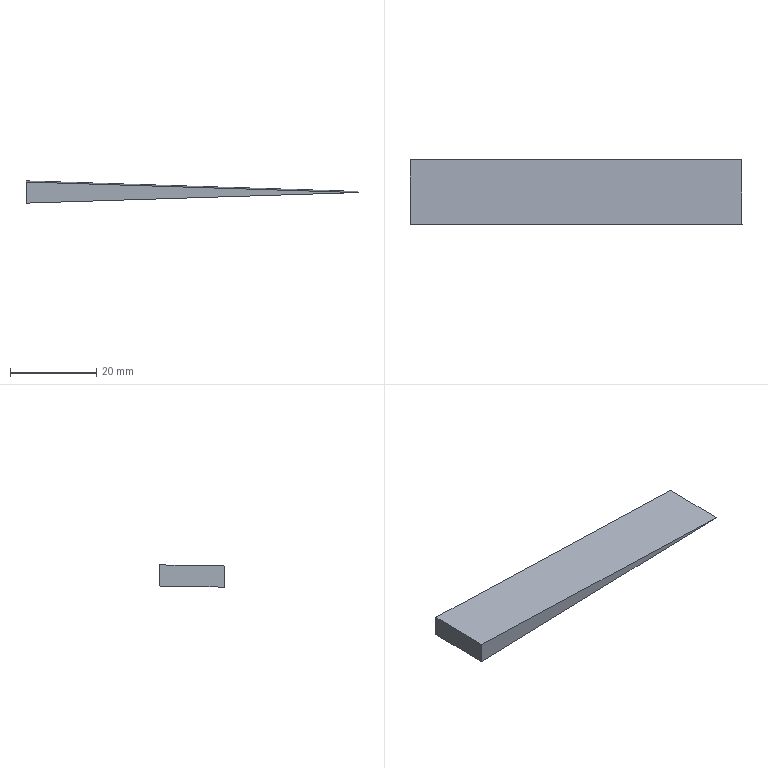Part | SolidWorks | features BaseBody 1 | 1 solid | 6 faces | box 77 x 15.083 x 5.155 mm | volume 2827 mm3 | plane 6
STEP:
#1=CARTESIAN_POINT('',(97.246,48.845,0.8517));
#2=VERTEX_POINT('',#1);
#3=CARTESIAN_POINT('',(97.246,48.845,0.8535));
#4=VERTEX_POINT('',#3);
#5=CARTESIAN_POINT('',(97.246,48.845,0.8526));
#6=DIRECTION('',(0.,-0.01745,0.9998));
#7=VECTOR('',#6,1000.);
#8=LINE('',#5,#7);
#9=EDGE_CURVE('',#2,#4,#8,.T.);
#10=ORIENTED_EDGE('',*,*,#9,.F.);
#11=CARTESIAN_POINT('',(97.245,63.843,1.113));
#12=VERTEX_POINT('',#11);
#13=CARTESIAN_POINT('',(97.246,48.845,0.8517));
#14=DIRECTION('',(-0.0000264,0.9998,0.01745));
#15=VECTOR('',#14,1000.);
#16=LINE('',#13,#15);
#17=EDGE_CURVE('',#2,#12,#16,.T.);
#18=ORIENTED_EDGE('',*,*,#17,.T.);
#19=CARTESIAN_POINT('',(97.245,63.843,1.115));
#20=VERTEX_POINT('',#19);
#21=CARTESIAN_POINT('',(97.245,63.843,1.114));
#22=DIRECTION('',(0.,-0.01745,0.9998));
#23=VECTOR('',#22,1000.);
#24=LINE('',#21,#23);
#25=EDGE_CURVE('',#12,#20,#24,.T.);
#26=ORIENTED_EDGE('',*,*,#25,.T.);
#27=CARTESIAN_POINT('',(97.245,63.843,1.115));
#28=DIRECTION('',(0.0000264,-0.9998,-0.01745));
#29=VECTOR('',#28,1000.);
#30=LINE('',#27,#29);
#31=EDGE_CURVE('',#20,#4,#30,.T.);
#32=ORIENTED_EDGE('',*,*,#31,.T.);
#33=EDGE_LOOP('',(#10,#18,#26,#32));
#34=FACE_OUTER_BOUND('',#33,.T.);
#35=CARTESIAN_POINT('',(97.246,48.755,0.8501));
#36=DIRECTION('',(1.,0.0000264,0.000000461));
#37=DIRECTION('',(-0.0000264,1.,0.));
#38=AXIS2_PLACEMENT_3D('',#35,#36,#37);
#39=PLANE('',#38);
#40=ADVANCED_FACE('',(#34),#39,.T.);
#41=ORIENTED_EDGE('',*,*,#17,.F.);
#42=CARTESIAN_POINT('',(20.246,48.886,-1.594));
#43=VERTEX_POINT('',#42);
#44=CARTESIAN_POINT('',(20.246,48.886,-1.594));
#45=DIRECTION('',(0.9995,-0.0005278,0.03175));
#46=VECTOR('',#45,1000.);
#47=LINE('',#44,#46);
#48=EDGE_CURVE('',#43,#2,#47,.T.);
#49=ORIENTED_EDGE('',*,*,#48,.F.);
#50=CARTESIAN_POINT('',(20.245,63.883,-1.332));
#51=VERTEX_POINT('',#50);
#52=CARTESIAN_POINT('',(20.245,63.883,-1.332));
#53=DIRECTION('',(0.0000264,-0.9998,-0.01745));
#54=VECTOR('',#53,1000.);
#55=LINE('',#52,#54);
#56=EDGE_CURVE('',#51,#43,#55,.T.);
#57=ORIENTED_EDGE('',*,*,#56,.F.);
#58=CARTESIAN_POINT('',(97.245,63.843,1.113));
#59=DIRECTION('',(-0.9995,0.0005278,-0.03175));
#60=VECTOR('',#59,1000.);
#61=LINE('',#58,#60);
#62=EDGE_CURVE('',#12,#51,#61,.T.);
#63=ORIENTED_EDGE('',*,*,#62,.F.);
#64=EDGE_LOOP('',(#41,#49,#57,#63));
#65=FACE_OUTER_BOUND('',#64,.T.);
#66=CARTESIAN_POINT('',(19.784,48.755,-1.611));
#67=DIRECTION('',(-0.03175,-0.01744,0.9993));
#68=DIRECTION('',(0.9995,0.,0.03176));
#69=AXIS2_PLACEMENT_3D('',#66,#67,#68);
#70=PLANE('',#69);
#71=ADVANCED_FACE('',(#65),#70,.F.);
#72=CARTESIAN_POINT('',(20.246,48.8,3.299));
#73=VERTEX_POINT('',#72);
#74=CARTESIAN_POINT('',(20.246,48.8,3.299));
#75=DIRECTION('',(0.9995,0.0005805,-0.03175));
#76=VECTOR('',#75,1000.);
#77=LINE('',#74,#76);
#78=EDGE_CURVE('',#73,#4,#77,.T.);
#79=ORIENTED_EDGE('',*,*,#78,.T.);
#80=ORIENTED_EDGE('',*,*,#31,.F.);
#81=CARTESIAN_POINT('',(20.245,63.798,3.561));
#82=VERTEX_POINT('',#81);
#83=CARTESIAN_POINT('',(97.245,63.843,1.115));
#84=DIRECTION('',(-0.9995,-0.0005805,0.03175));
#85=VECTOR('',#84,1000.);
#86=LINE('',#83,#85);
#87=EDGE_CURVE('',#20,#82,#86,.T.);
#88=ORIENTED_EDGE('',*,*,#87,.T.);
#89=CARTESIAN_POINT('',(20.245,63.798,3.561));
#90=DIRECTION('',(0.0000264,-0.9998,-0.01745));
#91=VECTOR('',#90,1000.);
#92=LINE('',#89,#91);
#93=EDGE_CURVE('',#82,#73,#92,.T.);
#94=ORIENTED_EDGE('',*,*,#93,.T.);
#95=EDGE_LOOP('',(#79,#80,#88,#94));
#96=FACE_OUTER_BOUND('',#95,.T.);
#97=CARTESIAN_POINT('',(19.775,48.71,3.313));
#98=DIRECTION('',(0.03175,-0.01744,0.9993));
#99=DIRECTION('',(0.9995,0.,-0.03176));
#100=AXIS2_PLACEMENT_3D('',#97,#98,#99);
#101=PLANE('',#100);
#102=ADVANCED_FACE('',(#96),#101,.T.);
#103=ORIENTED_EDGE('',*,*,#62,.T.);
#104=CARTESIAN_POINT('',(20.245,63.841,1.114));
#105=DIRECTION('',(0.,0.01745,-0.9998));
#106=VECTOR('',#105,1000.);
#107=LINE('',#104,#106);
#108=EDGE_CURVE('',#82,#51,#107,.T.);
#109=ORIENTED_EDGE('',*,*,#108,.F.);
#110=ORIENTED_EDGE('',*,*,#87,.F.);
#111=ORIENTED_EDGE('',*,*,#25,.F.);
#112=EDGE_LOOP('',(#103,#109,#110,#111));
#113=FACE_OUTER_BOUND('',#112,.T.);
#114=CARTESIAN_POINT('',(20.245,63.797,3.59));
#115=DIRECTION('',(0.0000264,-0.9998,-0.01745));
#116=DIRECTION('',(0.,0.01745,-0.9998));
#117=AXIS2_PLACEMENT_3D('',#114,#115,#116);
#118=PLANE('',#117);
#119=ADVANCED_FACE('',(#113),#118,.F.);
#120=CARTESIAN_POINT('',(20.246,48.843,0.8526));
#121=DIRECTION('',(0.,0.01745,-0.9998));
#122=VECTOR('',#121,1000.);
#123=LINE('',#120,#122);
#124=EDGE_CURVE('',#73,#43,#123,.T.);
#125=ORIENTED_EDGE('',*,*,#124,.T.);
#126=ORIENTED_EDGE('',*,*,#48,.T.);
#127=ORIENTED_EDGE('',*,*,#9,.T.);
#128=ORIENTED_EDGE('',*,*,#78,.F.);
#129=EDGE_LOOP('',(#125,#126,#127,#128));
#130=FACE_OUTER_BOUND('',#129,.T.);
#131=CARTESIAN_POINT('',(20.246,48.8,3.329));
#132=DIRECTION('',(0.0000264,-0.9998,-0.01745));
#133=DIRECTION('',(0.,0.01745,-0.9998));
#134=AXIS2_PLACEMENT_3D('',#131,#132,#133);
#135=PLANE('',#134);
#136=ADVANCED_FACE('',(#130),#135,.T.);
#137=ORIENTED_EDGE('',*,*,#124,.F.);
#138=ORIENTED_EDGE('',*,*,#93,.F.);
#139=ORIENTED_EDGE('',*,*,#108,.T.);
#140=ORIENTED_EDGE('',*,*,#56,.T.);
#141=EDGE_LOOP('',(#137,#138,#139,#140));
#142=FACE_OUTER_BOUND('',#141,.T.);
#143=CARTESIAN_POINT('',(20.245,63.974,-1.625));
#144=DIRECTION('',(-1.,-0.0000264,-0.000000461));
#145=DIRECTION('',(0.0000264,-1.,0.));
#146=AXIS2_PLACEMENT_3D('',#143,#144,#145);
#147=PLANE('',#146);
#148=ADVANCED_FACE('',(#142),#147,.T.);
#149=CLOSED_SHELL('',(#40,#71,#102,#119,#136,#148));
#150=MANIFOLD_SOLID_BREP('',#149);
#151=CARTESIAN_POINT('',(0.,0.,0.));
#152=DIRECTION('',(0.,0.,1.));
#153=DIRECTION('',(1.,0.,0.));
#154=AXIS2_PLACEMENT_3D('',#151,#152,#153);
#155=(LENGTH_UNIT()NAMED_UNIT(*)SI_UNIT(.MILLI.,.METRE.));
#156=UNCERTAINTY_MEASURE_WITH_UNIT(LENGTH_MEASURE(0.00001),#155,'','');
#157=(NAMED_UNIT(*)PLANE_ANGLE_UNIT()SI_UNIT($,.RADIAN.));
#158=(NAMED_UNIT(*)SI_UNIT($,.STERADIAN.)SOLID_ANGLE_UNIT());
#159=(GEOMETRIC_REPRESENTATION_CONTEXT(3)GLOBAL_UNCERTAINTY_ASSIGNED_CONTEXT((#156))GLOBAL_UNIT_ASSIGNED_CONTEXT((#155,#157,#158))REPRESENTATION_CONTEXT('',''));
#160=ADVANCED_BREP_SHAPE_REPRESENTATION('',(#150,#154),#159);